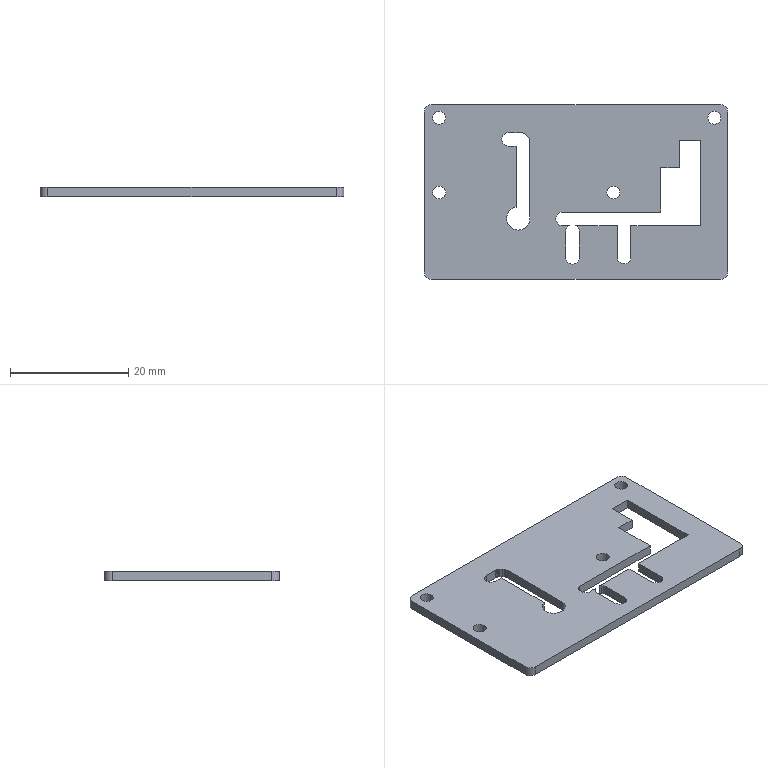Part | STEP file | VSWR protection control PCB | 1 solid | 65 faces | box 51.4 x 29.58 x 1.6 mm | volume 2088 mm3 | plane 53 | cylinder 12 | commonest cylinder face diameters 2.2 x4 2.54 x4 2.4 x2 2.312 x1 3.946 x1